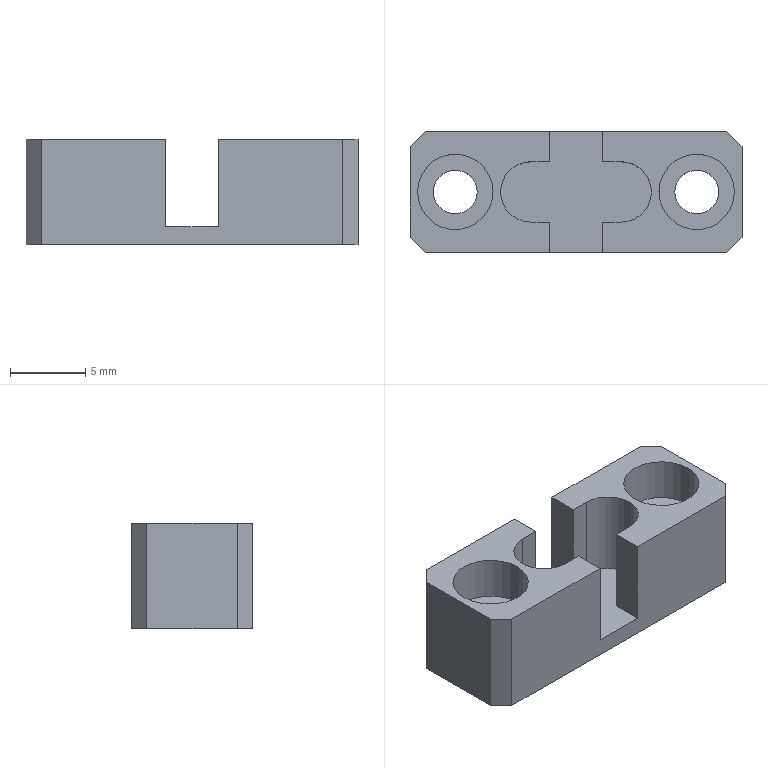Part | SolidWorks | features Chamfer 1, Extrusion 1, HoleWzd 1, ICE 1 | 1 solid | 33 faces | box 22 x 8 x 7 mm | volume 756.67 mm3 | plane 22 | cylinder 11 | commonest cylinder face diameters 2.9 x4 5 x4 4 x3
STEP:
#1=CARTESIAN_POINT('',(-10.5,0.,4.1));
#2=VERTEX_POINT('',#1);
#3=CARTESIAN_POINT('',(-5.5,0.,4.1));
#4=VERTEX_POINT('',#3);
#5=CARTESIAN_POINT('',(-8.,0.,4.1));
#6=DIRECTION('',(0.,0.,1.));
#7=DIRECTION('',(1.,0.,0.));
#8=AXIS2_PLACEMENT_3D('',#5,#6,#7);
#9=CIRCLE('',#8,2.5);
#10=EDGE_CURVE('',#2,#4,#9,.T.);
#11=ORIENTED_EDGE('',*,*,#10,.F.);
#12=CARTESIAN_POINT('',(-10.5,0.,7.));
#13=VERTEX_POINT('',#12);
#14=CARTESIAN_POINT('',(-10.5,0.,7.));
#15=DIRECTION('',(0.,0.,1.));
#16=VECTOR('',#15,1000.);
#17=LINE('',#14,#16);
#18=EDGE_CURVE('',#2,#13,#17,.T.);
#19=ORIENTED_EDGE('',*,*,#18,.T.);
#20=CARTESIAN_POINT('',(-5.5,0.,7.));
#21=VERTEX_POINT('',#20);
#22=CARTESIAN_POINT('',(-8.,0.,7.));
#23=DIRECTION('',(0.,0.,1.));
#24=DIRECTION('',(1.,0.,0.));
#25=AXIS2_PLACEMENT_3D('',#22,#23,#24);
#26=CIRCLE('',#25,2.5);
#27=EDGE_CURVE('',#13,#21,#26,.T.);
#28=ORIENTED_EDGE('',*,*,#27,.T.);
#29=CARTESIAN_POINT('',(-5.5,0.,7.));
#30=DIRECTION('',(0.,0.,1.));
#31=VECTOR('',#30,1000.);
#32=LINE('',#29,#31);
#33=EDGE_CURVE('',#4,#21,#32,.T.);
#34=ORIENTED_EDGE('',*,*,#33,.F.);
#35=EDGE_LOOP('',(#11,#19,#28,#34));
#36=FACE_OUTER_BOUND('',#35,.T.);
#37=CARTESIAN_POINT('',(-8.,0.,7.));
#38=DIRECTION('',(0.,0.,1.));
#39=DIRECTION('',(1.,0.,0.));
#40=AXIS2_PLACEMENT_3D('',#37,#38,#39);
#41=CYLINDRICAL_SURFACE('',#40,2.5);
#42=ADVANCED_FACE('',(#36),#41,.F.);
#43=CARTESIAN_POINT('',(-9.45,0.,0.));
#44=VERTEX_POINT('',#43);
#45=CARTESIAN_POINT('',(-6.55,0.,0.));
#46=VERTEX_POINT('',#45);
#47=CARTESIAN_POINT('',(-8.,0.,0.));
#48=DIRECTION('',(0.,0.,1.));
#49=DIRECTION('',(1.,0.,0.));
#50=AXIS2_PLACEMENT_3D('',#47,#48,#49);
#51=CIRCLE('',#50,1.45);
#52=EDGE_CURVE('',#44,#46,#51,.T.);
#53=ORIENTED_EDGE('',*,*,#52,.F.);
#54=CARTESIAN_POINT('',(-9.45,0.,4.1));
#55=VERTEX_POINT('',#54);
#56=CARTESIAN_POINT('',(-9.45,0.,7.));
#57=DIRECTION('',(0.,0.,1.));
#58=VECTOR('',#57,1000.);
#59=LINE('',#56,#58);
#60=EDGE_CURVE('',#44,#55,#59,.T.);
#61=ORIENTED_EDGE('',*,*,#60,.T.);
#62=CARTESIAN_POINT('',(-6.55,0.,4.1));
#63=VERTEX_POINT('',#62);
#64=CARTESIAN_POINT('',(-8.,0.,4.1));
#65=DIRECTION('',(0.,0.,1.));
#66=DIRECTION('',(1.,0.,0.));
#67=AXIS2_PLACEMENT_3D('',#64,#65,#66);
#68=CIRCLE('',#67,1.45);
#69=EDGE_CURVE('',#55,#63,#68,.T.);
#70=ORIENTED_EDGE('',*,*,#69,.T.);
#71=CARTESIAN_POINT('',(-6.55,0.,7.));
#72=DIRECTION('',(0.,0.,1.));
#73=VECTOR('',#72,1000.);
#74=LINE('',#71,#73);
#75=EDGE_CURVE('',#46,#63,#74,.T.);
#76=ORIENTED_EDGE('',*,*,#75,.F.);
#77=EDGE_LOOP('',(#53,#61,#70,#76));
#78=FACE_OUTER_BOUND('',#77,.T.);
#79=CARTESIAN_POINT('',(-8.,0.,7.));
#80=DIRECTION('',(0.,0.,1.));
#81=DIRECTION('',(1.,0.,0.));
#82=AXIS2_PLACEMENT_3D('',#79,#80,#81);
#83=CYLINDRICAL_SURFACE('',#82,1.45);
#84=ADVANCED_FACE('',(#78),#83,.F.);
#85=CARTESIAN_POINT('',(5.5,0.,4.1));
#86=VERTEX_POINT('',#85);
#87=CARTESIAN_POINT('',(10.5,0.,4.1));
#88=VERTEX_POINT('',#87);
#89=CARTESIAN_POINT('',(8.,0.,4.1));
#90=DIRECTION('',(0.,0.,1.));
#91=DIRECTION('',(1.,0.,0.));
#92=AXIS2_PLACEMENT_3D('',#89,#90,#91);
#93=CIRCLE('',#92,2.5);
#94=EDGE_CURVE('',#86,#88,#93,.T.);
#95=ORIENTED_EDGE('',*,*,#94,.F.);
#96=CARTESIAN_POINT('',(5.5,0.,7.));
#97=VERTEX_POINT('',#96);
#98=CARTESIAN_POINT('',(5.5,0.,7.));
#99=DIRECTION('',(0.,0.,1.));
#100=VECTOR('',#99,1000.);
#101=LINE('',#98,#100);
#102=EDGE_CURVE('',#86,#97,#101,.T.);
#103=ORIENTED_EDGE('',*,*,#102,.T.);
#104=CARTESIAN_POINT('',(10.5,0.,7.));
#105=VERTEX_POINT('',#104);
#106=CARTESIAN_POINT('',(8.,0.,7.));
#107=DIRECTION('',(0.,0.,1.));
#108=DIRECTION('',(1.,0.,0.));
#109=AXIS2_PLACEMENT_3D('',#106,#107,#108);
#110=CIRCLE('',#109,2.5);
#111=EDGE_CURVE('',#97,#105,#110,.T.);
#112=ORIENTED_EDGE('',*,*,#111,.T.);
#113=CARTESIAN_POINT('',(10.5,0.,7.));
#114=DIRECTION('',(0.,0.,1.));
#115=VECTOR('',#114,1000.);
#116=LINE('',#113,#115);
#117=EDGE_CURVE('',#88,#105,#116,.T.);
#118=ORIENTED_EDGE('',*,*,#117,.F.);
#119=EDGE_LOOP('',(#95,#103,#112,#118));
#120=FACE_OUTER_BOUND('',#119,.T.);
#121=CARTESIAN_POINT('',(8.,0.,7.));
#122=DIRECTION('',(0.,0.,1.));
#123=DIRECTION('',(1.,0.,0.));
#124=AXIS2_PLACEMENT_3D('',#121,#122,#123);
#125=CYLINDRICAL_SURFACE('',#124,2.5);
#126=ADVANCED_FACE('',(#120),#125,.F.);
#127=CARTESIAN_POINT('',(6.55,0.,0.));
#128=VERTEX_POINT('',#127);
#129=CARTESIAN_POINT('',(9.45,0.,0.));
#130=VERTEX_POINT('',#129);
#131=CARTESIAN_POINT('',(8.,0.,0.));
#132=DIRECTION('',(0.,0.,1.));
#133=DIRECTION('',(1.,0.,0.));
#134=AXIS2_PLACEMENT_3D('',#131,#132,#133);
#135=CIRCLE('',#134,1.45);
#136=EDGE_CURVE('',#128,#130,#135,.T.);
#137=ORIENTED_EDGE('',*,*,#136,.F.);
#138=CARTESIAN_POINT('',(6.55,0.,4.1));
#139=VERTEX_POINT('',#138);
#140=CARTESIAN_POINT('',(6.55,0.,7.));
#141=DIRECTION('',(0.,0.,1.));
#142=VECTOR('',#141,1000.);
#143=LINE('',#140,#142);
#144=EDGE_CURVE('',#128,#139,#143,.T.);
#145=ORIENTED_EDGE('',*,*,#144,.T.);
#146=CARTESIAN_POINT('',(9.45,0.,4.1));
#147=VERTEX_POINT('',#146);
#148=CARTESIAN_POINT('',(8.,0.,4.1));
#149=DIRECTION('',(0.,0.,1.));
#150=DIRECTION('',(1.,0.,0.));
#151=AXIS2_PLACEMENT_3D('',#148,#149,#150);
#152=CIRCLE('',#151,1.45);
#153=EDGE_CURVE('',#139,#147,#152,.T.);
#154=ORIENTED_EDGE('',*,*,#153,.T.);
#155=CARTESIAN_POINT('',(9.45,0.,7.));
#156=DIRECTION('',(0.,0.,1.));
#157=VECTOR('',#156,1000.);
#158=LINE('',#155,#157);
#159=EDGE_CURVE('',#130,#147,#158,.T.);
#160=ORIENTED_EDGE('',*,*,#159,.F.);
#161=EDGE_LOOP('',(#137,#145,#154,#160));
#162=FACE_OUTER_BOUND('',#161,.T.);
#163=CARTESIAN_POINT('',(8.,0.,7.));
#164=DIRECTION('',(0.,0.,1.));
#165=DIRECTION('',(1.,0.,0.));
#166=AXIS2_PLACEMENT_3D('',#163,#164,#165);
#167=CYLINDRICAL_SURFACE('',#166,1.45);
#168=ADVANCED_FACE('',(#162),#167,.F.);
#169=CARTESIAN_POINT('',(5.,0.,1.2));
#170=VERTEX_POINT('',#169);
#171=CARTESIAN_POINT('',(3.,2.,1.2));
#172=VERTEX_POINT('',#171);
#173=CARTESIAN_POINT('',(3.,0.,1.2));
#174=DIRECTION('',(0.,0.,1.));
#175=DIRECTION('',(-1.,0.,0.));
#176=AXIS2_PLACEMENT_3D('',#173,#174,#175);
#177=CIRCLE('',#176,2.);
#178=EDGE_CURVE('',#170,#172,#177,.T.);
#179=ORIENTED_EDGE('',*,*,#178,.F.);
#180=CARTESIAN_POINT('',(5.,0.,7.));
#181=VERTEX_POINT('',#180);
#182=CARTESIAN_POINT('',(5.,0.,1.2));
#183=DIRECTION('',(0.,0.,1.));
#184=VECTOR('',#183,1000.);
#185=LINE('',#182,#184);
#186=EDGE_CURVE('',#170,#181,#185,.T.);
#187=ORIENTED_EDGE('',*,*,#186,.T.);
#188=CARTESIAN_POINT('',(3.,2.,7.));
#189=VERTEX_POINT('',#188);
#190=CARTESIAN_POINT('',(3.,0.,7.));
#191=DIRECTION('',(0.,0.,1.));
#192=DIRECTION('',(-1.,0.,0.));
#193=AXIS2_PLACEMENT_3D('',#190,#191,#192);
#194=CIRCLE('',#193,2.);
#195=EDGE_CURVE('',#181,#189,#194,.T.);
#196=ORIENTED_EDGE('',*,*,#195,.T.);
#197=CARTESIAN_POINT('',(3.,2.,1.2));
#198=DIRECTION('',(0.,0.,1.));
#199=VECTOR('',#198,1000.);
#200=LINE('',#197,#199);
#201=EDGE_CURVE('',#172,#189,#200,.T.);
#202=ORIENTED_EDGE('',*,*,#201,.F.);
#203=EDGE_LOOP('',(#179,#187,#196,#202));
#204=FACE_OUTER_BOUND('',#203,.T.);
#205=CARTESIAN_POINT('',(3.,0.,1.2));
#206=DIRECTION('',(0.,0.,1.));
#207=DIRECTION('',(1.,0.,0.));
#208=AXIS2_PLACEMENT_3D('',#205,#206,#207);
#209=CYLINDRICAL_SURFACE('',#208,2.);
#210=ADVANCED_FACE('',(#204),#209,.F.);
#211=CARTESIAN_POINT('',(8.,0.,7.));
#212=DIRECTION('',(0.,0.,1.));
#213=DIRECTION('',(1.,0.,0.));
#214=AXIS2_PLACEMENT_3D('',#211,#212,#213);
#215=CIRCLE('',#214,2.5);
#216=EDGE_CURVE('',#105,#97,#215,.T.);
#217=ORIENTED_EDGE('',*,*,#216,.F.);
#218=ORIENTED_EDGE('',*,*,#111,.F.);
#219=EDGE_LOOP('',(#217,#218));
#220=FACE_BOUND('',#219,.T.);
#221=CARTESIAN_POINT('',(1.75,-4.,7.));
#222=VERTEX_POINT('',#221);
#223=CARTESIAN_POINT('',(10.,-4.,7.));
#224=VERTEX_POINT('',#223);
#225=CARTESIAN_POINT('',(-11.,-4.,7.));
#226=DIRECTION('',(1.,0.,0.));
#227=VECTOR('',#226,1000.);
#228=LINE('',#225,#227);
#229=EDGE_CURVE('',#222,#224,#228,.T.);
#230=ORIENTED_EDGE('',*,*,#229,.T.);
#231=CARTESIAN_POINT('',(11.,-3.,7.));
#232=VERTEX_POINT('',#231);
#233=CARTESIAN_POINT('',(11.,-3.,7.));
#234=DIRECTION('',(0.7071,0.7071,0.));
#235=VECTOR('',#234,1000.);
#236=LINE('',#233,#235);
#237=EDGE_CURVE('',#224,#232,#236,.T.);
#238=ORIENTED_EDGE('',*,*,#237,.T.);
#239=CARTESIAN_POINT('',(11.,3.,7.));
#240=VERTEX_POINT('',#239);
#241=CARTESIAN_POINT('',(11.,-4.,7.));
#242=DIRECTION('',(0.,1.,0.));
#243=VECTOR('',#242,1000.);
#244=LINE('',#241,#243);
#245=EDGE_CURVE('',#232,#240,#244,.T.);
#246=ORIENTED_EDGE('',*,*,#245,.T.);
#247=CARTESIAN_POINT('',(10.,4.,7.));
#248=VERTEX_POINT('',#247);
#249=CARTESIAN_POINT('',(10.,4.,7.));
#250=DIRECTION('',(-0.7071,0.7071,0.));
#251=VECTOR('',#250,1000.);
#252=LINE('',#249,#251);
#253=EDGE_CURVE('',#240,#248,#252,.T.);
#254=ORIENTED_EDGE('',*,*,#253,.T.);
#255=CARTESIAN_POINT('',(1.75,4.,7.));
#256=VERTEX_POINT('',#255);
#257=CARTESIAN_POINT('',(-11.,4.,7.));
#258=DIRECTION('',(-1.,0.,0.));
#259=VECTOR('',#258,1000.);
#260=LINE('',#257,#259);
#261=EDGE_CURVE('',#248,#256,#260,.T.);
#262=ORIENTED_EDGE('',*,*,#261,.T.);
#263=CARTESIAN_POINT('',(1.75,2.,7.));
#264=VERTEX_POINT('',#263);
#265=CARTESIAN_POINT('',(1.75,4.,7.));
#266=DIRECTION('',(0.,1.,0.));
#267=VECTOR('',#266,1000.);
#268=LINE('',#265,#267);
#269=EDGE_CURVE('',#264,#256,#268,.T.);
#270=ORIENTED_EDGE('',*,*,#269,.F.);
#271=CARTESIAN_POINT('',(1.75,2.,7.));
#272=DIRECTION('',(-1.,0.,0.));
#273=VECTOR('',#272,1000.);
#274=LINE('',#271,#273);
#275=EDGE_CURVE('',#189,#264,#274,.T.);
#276=ORIENTED_EDGE('',*,*,#275,.F.);
#277=ORIENTED_EDGE('',*,*,#195,.F.);
#278=CARTESIAN_POINT('',(3.,-2.,7.));
#279=VERTEX_POINT('',#278);
#280=CARTESIAN_POINT('',(3.,0.,7.));
#281=DIRECTION('',(0.,0.,1.));
#282=DIRECTION('',(-1.,0.,0.));
#283=AXIS2_PLACEMENT_3D('',#280,#281,#282);
#284=CIRCLE('',#283,2.);
#285=EDGE_CURVE('',#279,#181,#284,.T.);
#286=ORIENTED_EDGE('',*,*,#285,.F.);
#287=CARTESIAN_POINT('',(1.75,-2.,7.));
#288=VERTEX_POINT('',#287);
#289=CARTESIAN_POINT('',(1.75,-2.,7.));
#290=DIRECTION('',(1.,0.,0.));
#291=VECTOR('',#290,1000.);
#292=LINE('',#289,#291);
#293=EDGE_CURVE('',#288,#279,#292,.T.);
#294=ORIENTED_EDGE('',*,*,#293,.F.);
#295=CARTESIAN_POINT('',(1.75,-2.,7.));
#296=DIRECTION('',(0.,1.,0.));
#297=VECTOR('',#296,1000.);
#298=LINE('',#295,#297);
#299=EDGE_CURVE('',#222,#288,#298,.T.);
#300=ORIENTED_EDGE('',*,*,#299,.F.);
#301=EDGE_LOOP('',(#230,#238,#246,#254,#262,#270,#276,#277,#286,#294,#300));
#302=FACE_OUTER_BOUND('',#301,.T.);
#303=CARTESIAN_POINT('',(0.,0.,7.));
#304=DIRECTION('',(0.,0.,-1.));
#305=DIRECTION('',(-1.,0.,0.));
#306=AXIS2_PLACEMENT_3D('',#303,#304,#305);
#307=PLANE('',#306);
#308=ADVANCED_FACE('',(#220,#302),#307,.F.);
#309=ORIENTED_EDGE('',*,*,#245,.F.);
#310=CARTESIAN_POINT('',(11.,-3.,0.));
#311=VERTEX_POINT('',#310);
#312=CARTESIAN_POINT('',(11.,-3.,7.));
#313=DIRECTION('',(0.,0.,-1.));
#314=VECTOR('',#313,1000.);
#315=LINE('',#312,#314);
#316=EDGE_CURVE('',#232,#311,#315,.T.);
#317=ORIENTED_EDGE('',*,*,#316,.T.);
#318=CARTESIAN_POINT('',(11.,3.,0.));
#319=VERTEX_POINT('',#318);
#320=CARTESIAN_POINT('',(11.,-4.,0.));
#321=DIRECTION('',(0.,1.,0.));
#322=VECTOR('',#321,1000.);
#323=LINE('',#320,#322);
#324=EDGE_CURVE('',#311,#319,#323,.T.);
#325=ORIENTED_EDGE('',*,*,#324,.T.);
#326=CARTESIAN_POINT('',(11.,3.,7.));
#327=DIRECTION('',(0.,0.,1.));
#328=VECTOR('',#327,1000.);
#329=LINE('',#326,#328);
#330=EDGE_CURVE('',#319,#240,#329,.T.);
#331=ORIENTED_EDGE('',*,*,#330,.T.);
#332=EDGE_LOOP('',(#309,#317,#325,#331));
#333=FACE_OUTER_BOUND('',#332,.T.);
#334=CARTESIAN_POINT('',(11.,-4.,7.));
#335=DIRECTION('',(-1.,0.,0.));
#336=DIRECTION('',(0.,0.,1.));
#337=AXIS2_PLACEMENT_3D('',#334,#335,#336);
#338=PLANE('',#337);
#339=ADVANCED_FACE('',(#333),#338,.F.);
#340=ORIENTED_EDGE('',*,*,#261,.F.);
#341=CARTESIAN_POINT('',(10.,4.,0.));
#342=VERTEX_POINT('',#341);
#343=CARTESIAN_POINT('',(10.,4.,7.));
#344=DIRECTION('',(0.,0.,-1.));
#345=VECTOR('',#344,1000.);
#346=LINE('',#343,#345);
#347=EDGE_CURVE('',#248,#342,#346,.T.);
#348=ORIENTED_EDGE('',*,*,#347,.T.);
#349=CARTESIAN_POINT('',(-10.,4.,0.));
#350=VERTEX_POINT('',#349);
#351=CARTESIAN_POINT('',(-11.,4.,0.));
#352=DIRECTION('',(-1.,0.,0.));
#353=VECTOR('',#352,1000.);
#354=LINE('',#351,#353);
#355=EDGE_CURVE('',#342,#350,#354,.T.);
#356=ORIENTED_EDGE('',*,*,#355,.T.);
#357=CARTESIAN_POINT('',(-10.,4.,7.));
#358=VERTEX_POINT('',#357);
#359=CARTESIAN_POINT('',(-10.,4.,7.));
#360=DIRECTION('',(0.,0.,1.));
#361=VECTOR('',#360,1000.);
#362=LINE('',#359,#361);
#363=EDGE_CURVE('',#350,#358,#362,.T.);
#364=ORIENTED_EDGE('',*,*,#363,.T.);
#365=CARTESIAN_POINT('',(-1.75,4.,7.));
#366=VERTEX_POINT('',#365);
#367=CARTESIAN_POINT('',(-11.,4.,7.));
#368=DIRECTION('',(-1.,0.,0.));
#369=VECTOR('',#368,1000.);
#370=LINE('',#367,#369);
#371=EDGE_CURVE('',#366,#358,#370,.T.);
#372=ORIENTED_EDGE('',*,*,#371,.F.);
#373=CARTESIAN_POINT('',(-1.75,4.,1.2));
#374=VERTEX_POINT('',#373);
#375=CARTESIAN_POINT('',(-1.75,4.,1.2));
#376=DIRECTION('',(0.,0.,1.));
#377=VECTOR('',#376,1000.);
#378=LINE('',#375,#377);
#379=EDGE_CURVE('',#374,#366,#378,.T.);
#380=ORIENTED_EDGE('',*,*,#379,.F.);
#381=CARTESIAN_POINT('',(1.75,4.,1.2));
#382=VERTEX_POINT('',#381);
#383=CARTESIAN_POINT('',(-1.75,4.,1.2));
#384=DIRECTION('',(-1.,0.,0.));
#385=VECTOR('',#384,1000.);
#386=LINE('',#383,#385);
#387=EDGE_CURVE('',#382,#374,#386,.T.);
#388=ORIENTED_EDGE('',*,*,#387,.F.);
#389=CARTESIAN_POINT('',(1.75,4.,1.2));
#390=DIRECTION('',(0.,0.,1.));
#391=VECTOR('',#390,1000.);
#392=LINE('',#389,#391);
#393=EDGE_CURVE('',#382,#256,#392,.T.);
#394=ORIENTED_EDGE('',*,*,#393,.T.);
#395=EDGE_LOOP('',(#340,#348,#356,#364,#372,#380,#388,#394));
#396=FACE_OUTER_BOUND('',#395,.T.);
#397=CARTESIAN_POINT('',(-11.,4.,7.));
#398=DIRECTION('',(0.,-1.,0.));
#399=DIRECTION('',(0.,0.,-1.));
#400=AXIS2_PLACEMENT_3D('',#397,#398,#399);
#401=PLANE('',#400);
#402=ADVANCED_FACE('',(#396),#401,.F.);
#403=CARTESIAN_POINT('',(-11.,3.,0.));
#404=VERTEX_POINT('',#403);
#405=CARTESIAN_POINT('',(-11.,-3.,0.));
#406=VERTEX_POINT('',#405);
#407=CARTESIAN_POINT('',(-11.,-4.,0.));
#408=DIRECTION('',(0.,-1.,0.));
#409=VECTOR('',#408,1000.);
#410=LINE('',#407,#409);
#411=EDGE_CURVE('',#404,#406,#410,.T.);
#412=ORIENTED_EDGE('',*,*,#411,.T.);
#413=CARTESIAN_POINT('',(-11.,-3.,7.));
#414=VERTEX_POINT('',#413);
#415=CARTESIAN_POINT('',(-11.,-3.,7.));
#416=DIRECTION('',(0.,0.,1.));
#417=VECTOR('',#416,1000.);
#418=LINE('',#415,#417);
#419=EDGE_CURVE('',#406,#414,#418,.T.);
#420=ORIENTED_EDGE('',*,*,#419,.T.);
#421=CARTESIAN_POINT('',(-11.,3.,7.));
#422=VERTEX_POINT('',#421);
#423=CARTESIAN_POINT('',(-11.,-4.,7.));
#424=DIRECTION('',(0.,-1.,0.));
#425=VECTOR('',#424,1000.);
#426=LINE('',#423,#425);
#427=EDGE_CURVE('',#422,#414,#426,.T.);
#428=ORIENTED_EDGE('',*,*,#427,.F.);
#429=CARTESIAN_POINT('',(-11.,3.,7.));
#430=DIRECTION('',(0.,0.,-1.));
#431=VECTOR('',#430,1000.);
#432=LINE('',#429,#431);
#433=EDGE_CURVE('',#422,#404,#432,.T.);
#434=ORIENTED_EDGE('',*,*,#433,.T.);
#435=EDGE_LOOP('',(#412,#420,#428,#434));
#436=FACE_OUTER_BOUND('',#435,.T.);
#437=CARTESIAN_POINT('',(-11.,-4.,7.));
#438=DIRECTION('',(1.,0.,0.));
#439=DIRECTION('',(0.,0.,-1.));
#440=AXIS2_PLACEMENT_3D('',#437,#438,#439);
#441=PLANE('',#440);
#442=ADVANCED_FACE('',(#436),#441,.F.);
#443=CARTESIAN_POINT('',(-10.,-4.,0.));
#444=VERTEX_POINT('',#443);
#445=CARTESIAN_POINT('',(10.,-4.,0.));
#446=VERTEX_POINT('',#445);
#447=CARTESIAN_POINT('',(-11.,-4.,0.));
#448=DIRECTION('',(1.,0.,0.));
#449=VECTOR('',#448,1000.);
#450=LINE('',#447,#449);
#451=EDGE_CURVE('',#444,#446,#450,.T.);
#452=ORIENTED_EDGE('',*,*,#451,.T.);
#453=CARTESIAN_POINT('',(10.,-4.,7.));
#454=DIRECTION('',(0.,0.,1.));
#455=VECTOR('',#454,1000.);
#456=LINE('',#453,#455);
#457=EDGE_CURVE('',#446,#224,#456,.T.);
#458=ORIENTED_EDGE('',*,*,#457,.T.);
#459=ORIENTED_EDGE('',*,*,#229,.F.);
#460=CARTESIAN_POINT('',(1.75,-4.,1.2));
#461=VERTEX_POINT('',#460);
#462=CARTESIAN_POINT('',(1.75,-4.,1.2));
#463=DIRECTION('',(0.,0.,1.));
#464=VECTOR('',#463,1000.);
#465=LINE('',#462,#464);
#466=EDGE_CURVE('',#461,#222,#465,.T.);
#467=ORIENTED_EDGE('',*,*,#466,.F.);
#468=CARTESIAN_POINT('',(-1.75,-4.,1.2));
#469=VERTEX_POINT('',#468);
#470=CARTESIAN_POINT('',(-1.75,-4.,1.2));
#471=DIRECTION('',(1.,0.,0.));
#472=VECTOR('',#471,1000.);
#473=LINE('',#470,#472);
#474=EDGE_CURVE('',#469,#461,#473,.T.);
#475=ORIENTED_EDGE('',*,*,#474,.F.);
#476=CARTESIAN_POINT('',(-1.75,-4.,7.));
#477=VERTEX_POINT('',#476);
#478=CARTESIAN_POINT('',(-1.75,-4.,1.2));
#479=DIRECTION('',(0.,0.,1.));
#480=VECTOR('',#479,1000.);
#481=LINE('',#478,#480);
#482=EDGE_CURVE('',#469,#477,#481,.T.);
#483=ORIENTED_EDGE('',*,*,#482,.T.);
#484=CARTESIAN_POINT('',(-10.,-4.,7.));
#485=VERTEX_POINT('',#484);
#486=CARTESIAN_POINT('',(-11.,-4.,7.));
#487=DIRECTION('',(1.,0.,0.));
#488=VECTOR('',#487,1000.);
#489=LINE('',#486,#488);
#490=EDGE_CURVE('',#485,#477,#489,.T.);
#491=ORIENTED_EDGE('',*,*,#490,.F.);
#492=CARTESIAN_POINT('',(-10.,-4.,7.));
#493=DIRECTION('',(0.,0.,-1.));
#494=VECTOR('',#493,1000.);
#495=LINE('',#492,#494);
#496=EDGE_CURVE('',#485,#444,#495,.T.);
#497=ORIENTED_EDGE('',*,*,#496,.T.);
#498=EDGE_LOOP('',(#452,#458,#459,#467,#475,#483,#491,#497));
#499=FACE_OUTER_BOUND('',#498,.T.);
#500=CARTESIAN_POINT('',(-11.,-4.,7.));
#501=DIRECTION('',(0.,1.,0.));
#502=DIRECTION('',(0.,0.,1.));
#503=AXIS2_PLACEMENT_3D('',#500,#501,#502);
#504=PLANE('',#503);
#505=ADVANCED_FACE('',(#499),#504,.F.);
#506=CARTESIAN_POINT('',(-8.,0.,7.));
#507=DIRECTION('',(0.,0.,1.));
#508=DIRECTION('',(1.,0.,0.));
#509=AXIS2_PLACEMENT_3D('',#506,#507,#508);
#510=CIRCLE('',#509,2.5);
#511=EDGE_CURVE('',#21,#13,#510,.T.);
#512=ORIENTED_EDGE('',*,*,#511,.F.);
#513=ORIENTED_EDGE('',*,*,#27,.F.);
#514=EDGE_LOOP('',(#512,#513));
#515=FACE_BOUND('',#514,.T.);
#516=ORIENTED_EDGE('',*,*,#427,.T.);
#517=CARTESIAN_POINT('',(-10.,-4.,7.));
#518=DIRECTION('',(0.7071,-0.7071,0.));
#519=VECTOR('',#518,1000.);
#520=LINE('',#517,#519);
#521=EDGE_CURVE('',#414,#485,#520,.T.);
#522=ORIENTED_EDGE('',*,*,#521,.T.);
#523=ORIENTED_EDGE('',*,*,#490,.T.);
#524=CARTESIAN_POINT('',(-1.75,-2.,7.));
#525=VERTEX_POINT('',#524);
#526=CARTESIAN_POINT('',(-1.75,-2.,7.));
#527=DIRECTION('',(0.,-1.,0.));
#528=VECTOR('',#527,1000.);
#529=LINE('',#526,#528);
#530=EDGE_CURVE('',#525,#477,#529,.T.);
#531=ORIENTED_EDGE('',*,*,#530,.F.);
#532=CARTESIAN_POINT('',(-3.,-2.,7.));
#533=VERTEX_POINT('',#532);
#534=CARTESIAN_POINT('',(-3.,-2.,7.));
#535=DIRECTION('',(1.,0.,0.));
#536=VECTOR('',#535,1000.);
#537=LINE('',#534,#536);
#538=EDGE_CURVE('',#533,#525,#537,.T.);
#539=ORIENTED_EDGE('',*,*,#538,.F.);
#540=CARTESIAN_POINT('',(-3.,2.,7.));
#541=VERTEX_POINT('',#540);
#542=CARTESIAN_POINT('',(-3.,0.,7.));
#543=DIRECTION('',(0.,0.,1.));
#544=DIRECTION('',(1.,0.,0.));
#545=AXIS2_PLACEMENT_3D('',#542,#543,#544);
#546=CIRCLE('',#545,2.);
#547=EDGE_CURVE('',#541,#533,#546,.T.);
#548=ORIENTED_EDGE('',*,*,#547,.F.);
#549=CARTESIAN_POINT('',(-1.75,2.,7.));
#550=VERTEX_POINT('',#549);
#551=CARTESIAN_POINT('',(-3.,2.,7.));
#552=DIRECTION('',(-1.,0.,0.));
#553=VECTOR('',#552,1000.);
#554=LINE('',#551,#553);
#555=EDGE_CURVE('',#550,#541,#554,.T.);
#556=ORIENTED_EDGE('',*,*,#555,.F.);
#557=CARTESIAN_POINT('',(-1.75,4.,7.));
#558=DIRECTION('',(0.,-1.,0.));
#559=VECTOR('',#558,1000.);
#560=LINE('',#557,#559);
#561=EDGE_CURVE('',#366,#550,#560,.T.);
#562=ORIENTED_EDGE('',*,*,#561,.F.);
#563=ORIENTED_EDGE('',*,*,#371,.T.);
#564=CARTESIAN_POINT('',(-11.,3.,7.));
#565=DIRECTION('',(-0.7071,-0.7071,0.));
#566=VECTOR('',#565,1000.);
#567=LINE('',#564,#566);
#568=EDGE_CURVE('',#358,#422,#567,.T.);
#569=ORIENTED_EDGE('',*,*,#568,.T.);
#570=EDGE_LOOP('',(#516,#522,#523,#531,#539,#548,#556,#562,#563,#569));
#571=FACE_OUTER_BOUND('',#570,.T.);
#572=CARTESIAN_POINT('',(0.,0.,7.));
#573=DIRECTION('',(0.,0.,-1.));
#574=DIRECTION('',(-1.,0.,0.));
#575=AXIS2_PLACEMENT_3D('',#572,#573,#574);
#576=PLANE('',#575);
#577=ADVANCED_FACE('',(#515,#571),#576,.F.);
#578=CARTESIAN_POINT('',(-8.,0.,0.));
#579=DIRECTION('',(0.,0.,1.));
#580=DIRECTION('',(1.,0.,0.));
#581=AXIS2_PLACEMENT_3D('',#578,#579,#580);
#582=CIRCLE('',#581,1.45);
#583=EDGE_CURVE('',#46,#44,#582,.T.);
#584=ORIENTED_EDGE('',*,*,#583,.T.);
#585=ORIENTED_EDGE('',*,*,#52,.T.);
#586=EDGE_LOOP('',(#584,#585));
#587=FACE_BOUND('',#586,.T.);
#588=CARTESIAN_POINT('',(8.,0.,0.));
#589=DIRECTION('',(0.,0.,1.));
#590=DIRECTION('',(1.,0.,0.));
#591=AXIS2_PLACEMENT_3D('',#588,#589,#590);
#592=CIRCLE('',#591,1.45);
#593=EDGE_CURVE('',#130,#128,#592,.T.);
#594=ORIENTED_EDGE('',*,*,#593,.T.);
#595=ORIENTED_EDGE('',*,*,#136,.T.);
#596=EDGE_LOOP('',(#594,#595));
#597=FACE_BOUND('',#596,.T.);
#598=ORIENTED_EDGE('',*,*,#324,.F.);
#599=CARTESIAN_POINT('',(7.,-7.,0.));
#600=DIRECTION('',(-0.7071,-0.7071,0.));
#601=VECTOR('',#600,1000.);
#602=LINE('',#599,#601);
#603=EDGE_CURVE('',#311,#446,#602,.T.);
#604=ORIENTED_EDGE('',*,*,#603,.T.);
#605=ORIENTED_EDGE('',*,*,#451,.F.);
#606=CARTESIAN_POINT('',(-7.,-7.,0.));
#607=DIRECTION('',(-0.7071,0.7071,0.));
#608=VECTOR('',#607,1000.);
#609=LINE('',#606,#608);
#610=EDGE_CURVE('',#444,#406,#609,.T.);
#611=ORIENTED_EDGE('',*,*,#610,.T.);
#612=ORIENTED_EDGE('',*,*,#411,.F.);
#613=CARTESIAN_POINT('',(-7.,7.,0.));
#614=DIRECTION('',(0.7071,0.7071,0.));
#615=VECTOR('',#614,1000.);
#616=LINE('',#613,#615);
#617=EDGE_CURVE('',#404,#350,#616,.T.);
#618=ORIENTED_EDGE('',*,*,#617,.T.);
#619=ORIENTED_EDGE('',*,*,#355,.F.);
#620=CARTESIAN_POINT('',(7.,7.,0.));
#621=DIRECTION('',(0.7071,-0.7071,0.));
#622=VECTOR('',#621,1000.);
#623=LINE('',#620,#622);
#624=EDGE_CURVE('',#342,#319,#623,.T.);
#625=ORIENTED_EDGE('',*,*,#624,.T.);
#626=EDGE_LOOP('',(#598,#604,#605,#611,#612,#618,#619,#625));
#627=FACE_OUTER_BOUND('',#626,.T.);
#628=CARTESIAN_POINT('',(0.,0.,0.));
#629=DIRECTION('',(0.,0.,-1.));
#630=DIRECTION('',(-1.,0.,0.));
#631=AXIS2_PLACEMENT_3D('',#628,#629,#630);
#632=PLANE('',#631);
#633=ADVANCED_FACE('',(#587,#597,#627),#632,.T.);
#634=ORIENTED_EDGE('',*,*,#561,.T.);
#635=CARTESIAN_POINT('',(-1.75,2.,1.2));
#636=VERTEX_POINT('',#635);
#637=CARTESIAN_POINT('',(-1.75,2.,1.2));
#638=DIRECTION('',(0.,0.,1.));
#639=VECTOR('',#638,1000.);
#640=LINE('',#637,#639);
#641=EDGE_CURVE('',#636,#550,#640,.T.);
#642=ORIENTED_EDGE('',*,*,#641,.F.);
#643=CARTESIAN_POINT('',(-1.75,4.,1.2));
#644=DIRECTION('',(0.,-1.,0.));
#645=VECTOR('',#644,1000.);
#646=LINE('',#643,#645);
#647=EDGE_CURVE('',#374,#636,#646,.T.);
#648=ORIENTED_EDGE('',*,*,#647,.F.);
#649=ORIENTED_EDGE('',*,*,#379,.T.);
#650=EDGE_LOOP('',(#634,#642,#648,#649));
#651=FACE_OUTER_BOUND('',#650,.T.);
#652=CARTESIAN_POINT('',(-1.75,4.,1.2));
#653=DIRECTION('',(-1.,0.,0.));
#654=DIRECTION('',(0.,-1.,0.));
#655=AXIS2_PLACEMENT_3D('',#652,#653,#654);
#656=PLANE('',#655);
#657=ADVANCED_FACE('',(#651),#656,.F.);
#658=ORIENTED_EDGE('',*,*,#269,.T.);
#659=ORIENTED_EDGE('',*,*,#393,.F.);
#660=CARTESIAN_POINT('',(1.75,2.,1.2));
#661=VERTEX_POINT('',#660);
#662=CARTESIAN_POINT('',(1.75,4.,1.2));
#663=DIRECTION('',(0.,1.,0.));
#664=VECTOR('',#663,1000.);
#665=LINE('',#662,#664);
#666=EDGE_CURVE('',#661,#382,#665,.T.);
#667=ORIENTED_EDGE('',*,*,#666,.F.);
#668=CARTESIAN_POINT('',(1.75,2.,1.2));
#669=DIRECTION('',(0.,0.,1.));
#670=VECTOR('',#669,1000.);
#671=LINE('',#668,#670);
#672=EDGE_CURVE('',#661,#264,#671,.T.);
#673=ORIENTED_EDGE('',*,*,#672,.T.);
#674=EDGE_LOOP('',(#658,#659,#667,#673));
#675=FACE_OUTER_BOUND('',#674,.T.);
#676=CARTESIAN_POINT('',(1.75,4.,1.2));
#677=DIRECTION('',(1.,0.,0.));
#678=DIRECTION('',(0.,1.,0.));
#679=AXIS2_PLACEMENT_3D('',#676,#677,#678);
#680=PLANE('',#679);
#681=ADVANCED_FACE('',(#675),#680,.F.);
#682=ORIENTED_EDGE('',*,*,#275,.T.);
#683=ORIENTED_EDGE('',*,*,#672,.F.);
#684=CARTESIAN_POINT('',(1.75,2.,1.2));
#685=DIRECTION('',(-1.,0.,0.));
#686=VECTOR('',#685,1000.);
#687=LINE('',#684,#686);
#688=EDGE_CURVE('',#172,#661,#687,.T.);
#689=ORIENTED_EDGE('',*,*,#688,.F.);
#690=ORIENTED_EDGE('',*,*,#201,.T.);
#691=EDGE_LOOP('',(#682,#683,#689,#690));
#692=FACE_OUTER_BOUND('',#691,.T.);
#693=CARTESIAN_POINT('',(1.75,2.,1.2));
#694=DIRECTION('',(0.,1.,0.));
#695=DIRECTION('',(-1.,0.,0.));
#696=AXIS2_PLACEMENT_3D('',#693,#694,#695);
#697=PLANE('',#696);
#698=ADVANCED_FACE('',(#692),#697,.F.);
#699=ORIENTED_EDGE('',*,*,#186,.F.);
#700=CARTESIAN_POINT('',(3.,-2.,1.2));
#701=VERTEX_POINT('',#700);
#702=CARTESIAN_POINT('',(3.,0.,1.2));
#703=DIRECTION('',(0.,0.,1.));
#704=DIRECTION('',(-1.,0.,0.));
#705=AXIS2_PLACEMENT_3D('',#702,#703,#704);
#706=CIRCLE('',#705,2.);
#707=EDGE_CURVE('',#701,#170,#706,.T.);
#708=ORIENTED_EDGE('',*,*,#707,.F.);
#709=CARTESIAN_POINT('',(3.,-2.,1.2));
#710=DIRECTION('',(0.,0.,1.));
#711=VECTOR('',#710,1000.);
#712=LINE('',#709,#711);
#713=EDGE_CURVE('',#701,#279,#712,.T.);
#714=ORIENTED_EDGE('',*,*,#713,.T.);
#715=ORIENTED_EDGE('',*,*,#285,.T.);
#716=EDGE_LOOP('',(#699,#708,#714,#715));
#717=FACE_OUTER_BOUND('',#716,.T.);
#718=CARTESIAN_POINT('',(3.,0.,1.2));
#719=DIRECTION('',(0.,0.,1.));
#720=DIRECTION('',(1.,0.,0.));
#721=AXIS2_PLACEMENT_3D('',#718,#719,#720);
#722=CYLINDRICAL_SURFACE('',#721,2.);
#723=ADVANCED_FACE('',(#717),#722,.F.);
#724=ORIENTED_EDGE('',*,*,#293,.T.);
#725=ORIENTED_EDGE('',*,*,#713,.F.);
#726=CARTESIAN_POINT('',(1.75,-2.,1.2));
#727=VERTEX_POINT('',#726);
#728=CARTESIAN_POINT('',(1.75,-2.,1.2));
#729=DIRECTION('',(1.,0.,0.));
#730=VECTOR('',#729,1000.);
#731=LINE('',#728,#730);
#732=EDGE_CURVE('',#727,#701,#731,.T.);
#733=ORIENTED_EDGE('',*,*,#732,.F.);
#734=CARTESIAN_POINT('',(1.75,-2.,1.2));
#735=DIRECTION('',(0.,0.,1.));
#736=VECTOR('',#735,1000.);
#737=LINE('',#734,#736);
#738=EDGE_CURVE('',#727,#288,#737,.T.);
#739=ORIENTED_EDGE('',*,*,#738,.T.);
#740=EDGE_LOOP('',(#724,#725,#733,#739));
#741=FACE_OUTER_BOUND('',#740,.T.);
#742=CARTESIAN_POINT('',(1.75,-2.,1.2));
#743=DIRECTION('',(0.,-1.,0.));
#744=DIRECTION('',(1.,0.,0.));
#745=AXIS2_PLACEMENT_3D('',#742,#743,#744);
#746=PLANE('',#745);
#747=ADVANCED_FACE('',(#741),#746,.F.);
#748=ORIENTED_EDGE('',*,*,#299,.T.);
#749=ORIENTED_EDGE('',*,*,#738,.F.);
#750=CARTESIAN_POINT('',(1.75,-2.,1.2));
#751=DIRECTION('',(0.,1.,0.));
#752=VECTOR('',#751,1000.);
#753=LINE('',#750,#752);
#754=EDGE_CURVE('',#461,#727,#753,.T.);
#755=ORIENTED_EDGE('',*,*,#754,.F.);
#756=ORIENTED_EDGE('',*,*,#466,.T.);
#757=EDGE_LOOP('',(#748,#749,#755,#756));
#758=FACE_OUTER_BOUND('',#757,.T.);
#759=CARTESIAN_POINT('',(1.75,-2.,1.2));
#760=DIRECTION('',(1.,0.,0.));
#761=DIRECTION('',(0.,1.,0.));
#762=AXIS2_PLACEMENT_3D('',#759,#760,#761);
#763=PLANE('',#762);
#764=ADVANCED_FACE('',(#758),#763,.F.);
#765=ORIENTED_EDGE('',*,*,#530,.T.);
#766=ORIENTED_EDGE('',*,*,#482,.F.);
#767=CARTESIAN_POINT('',(-1.75,-2.,1.2));
#768=VERTEX_POINT('',#767);
#769=CARTESIAN_POINT('',(-1.75,-2.,1.2));
#770=DIRECTION('',(0.,-1.,0.));
#771=VECTOR('',#770,1000.);
#772=LINE('',#769,#771);
#773=EDGE_CURVE('',#768,#469,#772,.T.);
#774=ORIENTED_EDGE('',*,*,#773,.F.);
#775=CARTESIAN_POINT('',(-1.75,-2.,1.2));
#776=DIRECTION('',(0.,0.,1.));
#777=VECTOR('',#776,1000.);
#778=LINE('',#775,#777);
#779=EDGE_CURVE('',#768,#525,#778,.T.);
#780=ORIENTED_EDGE('',*,*,#779,.T.);
#781=EDGE_LOOP('',(#765,#766,#774,#780));
#782=FACE_OUTER_BOUND('',#781,.T.);
#783=CARTESIAN_POINT('',(-1.75,-2.,1.2));
#784=DIRECTION('',(-1.,0.,0.));
#785=DIRECTION('',(0.,-1.,0.));
#786=AXIS2_PLACEMENT_3D('',#783,#784,#785);
#787=PLANE('',#786);
#788=ADVANCED_FACE('',(#782),#787,.F.);
#789=ORIENTED_EDGE('',*,*,#538,.T.);
#790=ORIENTED_EDGE('',*,*,#779,.F.);
#791=CARTESIAN_POINT('',(-3.,-2.,1.2));
#792=VERTEX_POINT('',#791);
#793=CARTESIAN_POINT('',(-3.,-2.,1.2));
#794=DIRECTION('',(1.,0.,0.));
#795=VECTOR('',#794,1000.);
#796=LINE('',#793,#795);
#797=EDGE_CURVE('',#792,#768,#796,.T.);
#798=ORIENTED_EDGE('',*,*,#797,.F.);
#799=CARTESIAN_POINT('',(-3.,-2.,1.2));
#800=DIRECTION('',(0.,0.,1.));
#801=VECTOR('',#800,1000.);
#802=LINE('',#799,#801);
#803=EDGE_CURVE('',#792,#533,#802,.T.);
#804=ORIENTED_EDGE('',*,*,#803,.T.);
#805=EDGE_LOOP('',(#789,#790,#798,#804));
#806=FACE_OUTER_BOUND('',#805,.T.);
#807=CARTESIAN_POINT('',(-3.,-2.,1.2));
#808=DIRECTION('',(0.,-1.,0.));
#809=DIRECTION('',(0.,0.,-1.));
#810=AXIS2_PLACEMENT_3D('',#807,#808,#809);
#811=PLANE('',#810);
#812=ADVANCED_FACE('',(#806),#811,.F.);
#813=ORIENTED_EDGE('',*,*,#547,.T.);
#814=ORIENTED_EDGE('',*,*,#803,.F.);
#815=CARTESIAN_POINT('',(-3.,2.,1.2));
#816=VERTEX_POINT('',#815);
#817=CARTESIAN_POINT('',(-3.,0.,1.2));
#818=DIRECTION('',(0.,0.,1.));
#819=DIRECTION('',(1.,0.,0.));
#820=AXIS2_PLACEMENT_3D('',#817,#818,#819);
#821=CIRCLE('',#820,2.);
#822=EDGE_CURVE('',#816,#792,#821,.T.);
#823=ORIENTED_EDGE('',*,*,#822,.F.);
#824=CARTESIAN_POINT('',(-3.,2.,1.2));
#825=DIRECTION('',(0.,0.,1.));
#826=VECTOR('',#825,1000.);
#827=LINE('',#824,#826);
#828=EDGE_CURVE('',#816,#541,#827,.T.);
#829=ORIENTED_EDGE('',*,*,#828,.T.);
#830=EDGE_LOOP('',(#813,#814,#823,#829));
#831=FACE_OUTER_BOUND('',#830,.T.);
#832=CARTESIAN_POINT('',(-3.,0.,1.2));
#833=DIRECTION('',(0.,0.,1.));
#834=DIRECTION('',(1.,0.,0.));
#835=AXIS2_PLACEMENT_3D('',#832,#833,#834);
#836=CYLINDRICAL_SURFACE('',#835,2.);
#837=ADVANCED_FACE('',(#831),#836,.F.);
#838=ORIENTED_EDGE('',*,*,#555,.T.);
#839=ORIENTED_EDGE('',*,*,#828,.F.);
#840=CARTESIAN_POINT('',(-3.,2.,1.2));
#841=DIRECTION('',(-1.,0.,0.));
#842=VECTOR('',#841,1000.);
#843=LINE('',#840,#842);
#844=EDGE_CURVE('',#636,#816,#843,.T.);
#845=ORIENTED_EDGE('',*,*,#844,.F.);
#846=ORIENTED_EDGE('',*,*,#641,.T.);
#847=EDGE_LOOP('',(#838,#839,#845,#846));
#848=FACE_OUTER_BOUND('',#847,.T.);
#849=CARTESIAN_POINT('',(-3.,2.,1.2));
#850=DIRECTION('',(0.,1.,0.));
#851=DIRECTION('',(0.,0.,1.));
#852=AXIS2_PLACEMENT_3D('',#849,#850,#851);
#853=PLANE('',#852);
#854=ADVANCED_FACE('',(#848),#853,.F.);
#855=ORIENTED_EDGE('',*,*,#647,.T.);
#856=ORIENTED_EDGE('',*,*,#844,.T.);
#857=ORIENTED_EDGE('',*,*,#822,.T.);
#858=ORIENTED_EDGE('',*,*,#797,.T.);
#859=ORIENTED_EDGE('',*,*,#773,.T.);
#860=ORIENTED_EDGE('',*,*,#474,.T.);
#861=ORIENTED_EDGE('',*,*,#754,.T.);
#862=ORIENTED_EDGE('',*,*,#732,.T.);
#863=ORIENTED_EDGE('',*,*,#707,.T.);
#864=ORIENTED_EDGE('',*,*,#178,.T.);
#865=ORIENTED_EDGE('',*,*,#688,.T.);
#866=ORIENTED_EDGE('',*,*,#666,.T.);
#867=ORIENTED_EDGE('',*,*,#387,.T.);
#868=EDGE_LOOP('',(#855,#856,#857,#858,#859,#860,#861,#862,#863,#864,#865,#866,#867));
#869=FACE_OUTER_BOUND('',#868,.T.);
#870=CARTESIAN_POINT('',(-3.,0.,1.2));
#871=DIRECTION('',(0.,0.,1.));
#872=DIRECTION('',(1.,0.,0.));
#873=AXIS2_PLACEMENT_3D('',#870,#871,#872);
#874=PLANE('',#873);
#875=ADVANCED_FACE('',(#869),#874,.T.);
#876=ORIENTED_EDGE('',*,*,#237,.F.);
#877=ORIENTED_EDGE('',*,*,#457,.F.);
#878=ORIENTED_EDGE('',*,*,#603,.F.);
#879=ORIENTED_EDGE('',*,*,#316,.F.);
#880=EDGE_LOOP('',(#876,#877,#878,#879));
#881=FACE_OUTER_BOUND('',#880,.T.);
#882=CARTESIAN_POINT('',(11.,-3.,7.));
#883=DIRECTION('',(-0.7071,0.7071,0.));
#884=DIRECTION('',(0.,0.,-1.));
#885=AXIS2_PLACEMENT_3D('',#882,#883,#884);
#886=PLANE('',#885);
#887=ADVANCED_FACE('',(#881),#886,.F.);
#888=ORIENTED_EDGE('',*,*,#253,.F.);
#889=ORIENTED_EDGE('',*,*,#330,.F.);
#890=ORIENTED_EDGE('',*,*,#624,.F.);
#891=ORIENTED_EDGE('',*,*,#347,.F.);
#892=EDGE_LOOP('',(#888,#889,#890,#891));
#893=FACE_OUTER_BOUND('',#892,.T.);
#894=CARTESIAN_POINT('',(10.,4.,7.));
#895=DIRECTION('',(-0.7071,-0.7071,0.));
#896=DIRECTION('',(0.,0.,-1.));
#897=AXIS2_PLACEMENT_3D('',#894,#895,#896);
#898=PLANE('',#897);
#899=ADVANCED_FACE('',(#893),#898,.F.);
#900=ORIENTED_EDGE('',*,*,#521,.F.);
#901=ORIENTED_EDGE('',*,*,#419,.F.);
#902=ORIENTED_EDGE('',*,*,#610,.F.);
#903=ORIENTED_EDGE('',*,*,#496,.F.);
#904=EDGE_LOOP('',(#900,#901,#902,#903));
#905=FACE_OUTER_BOUND('',#904,.T.);
#906=CARTESIAN_POINT('',(-10.,-4.,7.));
#907=DIRECTION('',(0.7071,0.7071,0.));
#908=DIRECTION('',(0.,0.,-1.));
#909=AXIS2_PLACEMENT_3D('',#906,#907,#908);
#910=PLANE('',#909);
#911=ADVANCED_FACE('',(#905),#910,.F.);
#912=ORIENTED_EDGE('',*,*,#568,.F.);
#913=ORIENTED_EDGE('',*,*,#363,.F.);
#914=ORIENTED_EDGE('',*,*,#617,.F.);
#915=ORIENTED_EDGE('',*,*,#433,.F.);
#916=EDGE_LOOP('',(#912,#913,#914,#915));
#917=FACE_OUTER_BOUND('',#916,.T.);
#918=CARTESIAN_POINT('',(-11.,3.,7.));
#919=DIRECTION('',(0.7071,-0.7071,0.));
#920=DIRECTION('',(0.,0.,-1.));
#921=AXIS2_PLACEMENT_3D('',#918,#919,#920);
#922=PLANE('',#921);
#923=ADVANCED_FACE('',(#917),#922,.F.);
#924=ORIENTED_EDGE('',*,*,#144,.F.);
#925=ORIENTED_EDGE('',*,*,#593,.F.);
#926=ORIENTED_EDGE('',*,*,#159,.T.);
#927=CARTESIAN_POINT('',(8.,0.,4.1));
#928=DIRECTION('',(0.,0.,1.));
#929=DIRECTION('',(1.,0.,0.));
#930=AXIS2_PLACEMENT_3D('',#927,#928,#929);
#931=CIRCLE('',#930,1.45);
#932=EDGE_CURVE('',#147,#139,#931,.T.);
#933=ORIENTED_EDGE('',*,*,#932,.T.);
#934=EDGE_LOOP('',(#924,#925,#926,#933));
#935=FACE_OUTER_BOUND('',#934,.T.);
#936=CARTESIAN_POINT('',(8.,0.,7.));
#937=DIRECTION('',(0.,0.,1.));
#938=DIRECTION('',(1.,0.,0.));
#939=AXIS2_PLACEMENT_3D('',#936,#937,#938);
#940=CYLINDRICAL_SURFACE('',#939,1.45);
#941=ADVANCED_FACE('',(#935),#940,.F.);
#942=ORIENTED_EDGE('',*,*,#932,.F.);
#943=ORIENTED_EDGE('',*,*,#153,.F.);
#944=EDGE_LOOP('',(#942,#943));
#945=FACE_BOUND('',#944,.T.);
#946=CARTESIAN_POINT('',(8.,0.,4.1));
#947=DIRECTION('',(0.,0.,1.));
#948=DIRECTION('',(1.,0.,0.));
#949=AXIS2_PLACEMENT_3D('',#946,#947,#948);
#950=CIRCLE('',#949,2.5);
#951=EDGE_CURVE('',#88,#86,#950,.T.);
#952=ORIENTED_EDGE('',*,*,#951,.T.);
#953=ORIENTED_EDGE('',*,*,#94,.T.);
#954=EDGE_LOOP('',(#952,#953));
#955=FACE_OUTER_BOUND('',#954,.T.);
#956=CARTESIAN_POINT('',(9.45,0.,4.1));
#957=DIRECTION('',(0.,0.,-1.));
#958=DIRECTION('',(-1.,0.,0.));
#959=AXIS2_PLACEMENT_3D('',#956,#957,#958);
#960=PLANE('',#959);
#961=ADVANCED_FACE('',(#945,#955),#960,.F.);
#962=ORIENTED_EDGE('',*,*,#102,.F.);
#963=ORIENTED_EDGE('',*,*,#951,.F.);
#964=ORIENTED_EDGE('',*,*,#117,.T.);
#965=ORIENTED_EDGE('',*,*,#216,.T.);
#966=EDGE_LOOP('',(#962,#963,#964,#965));
#967=FACE_OUTER_BOUND('',#966,.T.);
#968=CARTESIAN_POINT('',(8.,0.,7.));
#969=DIRECTION('',(0.,0.,1.));
#970=DIRECTION('',(1.,0.,0.));
#971=AXIS2_PLACEMENT_3D('',#968,#969,#970);
#972=CYLINDRICAL_SURFACE('',#971,2.5);
#973=ADVANCED_FACE('',(#967),#972,.F.);
#974=ORIENTED_EDGE('',*,*,#60,.F.);
#975=ORIENTED_EDGE('',*,*,#583,.F.);
#976=ORIENTED_EDGE('',*,*,#75,.T.);
#977=CARTESIAN_POINT('',(-8.,0.,4.1));
#978=DIRECTION('',(0.,0.,1.));
#979=DIRECTION('',(1.,0.,0.));
#980=AXIS2_PLACEMENT_3D('',#977,#978,#979);
#981=CIRCLE('',#980,1.45);
#982=EDGE_CURVE('',#63,#55,#981,.T.);
#983=ORIENTED_EDGE('',*,*,#982,.T.);
#984=EDGE_LOOP('',(#974,#975,#976,#983));
#985=FACE_OUTER_BOUND('',#984,.T.);
#986=CARTESIAN_POINT('',(-8.,0.,7.));
#987=DIRECTION('',(0.,0.,1.));
#988=DIRECTION('',(1.,0.,0.));
#989=AXIS2_PLACEMENT_3D('',#986,#987,#988);
#990=CYLINDRICAL_SURFACE('',#989,1.45);
#991=ADVANCED_FACE('',(#985),#990,.F.);
#992=ORIENTED_EDGE('',*,*,#982,.F.);
#993=ORIENTED_EDGE('',*,*,#69,.F.);
#994=EDGE_LOOP('',(#992,#993));
#995=FACE_BOUND('',#994,.T.);
#996=CARTESIAN_POINT('',(-8.,0.,4.1));
#997=DIRECTION('',(0.,0.,1.));
#998=DIRECTION('',(1.,0.,0.));
#999=AXIS2_PLACEMENT_3D('',#996,#997,#998);
#1000=CIRCLE('',#999,2.5);
#1001=EDGE_CURVE('',#4,#2,#1000,.T.);
#1002=ORIENTED_EDGE('',*,*,#1001,.T.);
#1003=ORIENTED_EDGE('',*,*,#10,.T.);
#1004=EDGE_LOOP('',(#1002,#1003));
#1005=FACE_OUTER_BOUND('',#1004,.T.);
#1006=CARTESIAN_POINT('',(-6.55,0.,4.1));
#1007=DIRECTION('',(0.,0.,-1.));
#1008=DIRECTION('',(-1.,0.,0.));
#1009=AXIS2_PLACEMENT_3D('',#1006,#1007,#1008);
#1010=PLANE('',#1009);
#1011=ADVANCED_FACE('',(#995,#1005),#1010,.F.);
#1012=ORIENTED_EDGE('',*,*,#18,.F.);
#1013=ORIENTED_EDGE('',*,*,#1001,.F.);
#1014=ORIENTED_EDGE('',*,*,#33,.T.);
#1015=ORIENTED_EDGE('',*,*,#511,.T.);
#1016=EDGE_LOOP('',(#1012,#1013,#1014,#1015));
#1017=FACE_OUTER_BOUND('',#1016,.T.);
#1018=CARTESIAN_POINT('',(-8.,0.,7.));
#1019=DIRECTION('',(0.,0.,1.));
#1020=DIRECTION('',(1.,0.,0.));
#1021=AXIS2_PLACEMENT_3D('',#1018,#1019,#1020);
#1022=CYLINDRICAL_SURFACE('',#1021,2.5);
#1023=ADVANCED_FACE('',(#1017),#1022,.F.);
#1024=CLOSED_SHELL('',(#42,#84,#126,#168,#210,#308,#339,#402,#442,#505,#577,#633,#657,#681,#698,#723,#747,#764,#788,#812,#837,#854,#875,#887,#899,#911,#923,#941,#961,#973,#991,#1011,#1023));
#1025=MANIFOLD_SOLID_BREP('',#1024);
#1026=CARTESIAN_POINT('',(0.,0.,0.));
#1027=DIRECTION('',(0.,0.,1.));
#1028=DIRECTION('',(1.,0.,0.));
#1029=AXIS2_PLACEMENT_3D('',#1026,#1027,#1028);
#1030=(LENGTH_UNIT()NAMED_UNIT(*)SI_UNIT(.MILLI.,.METRE.));
#1031=UNCERTAINTY_MEASURE_WITH_UNIT(LENGTH_MEASURE(0.00001),#1030,'','');
#1032=(NAMED_UNIT(*)PLANE_ANGLE_UNIT()SI_UNIT($,.RADIAN.));
#1033=(NAMED_UNIT(*)SI_UNIT($,.STERADIAN.)SOLID_ANGLE_UNIT());
#1034=(GEOMETRIC_REPRESENTATION_CONTEXT(3)GLOBAL_UNCERTAINTY_ASSIGNED_CONTEXT((#1031))GLOBAL_UNIT_ASSIGNED_CONTEXT((#1030,#1032,#1033))REPRESENTATION_CONTEXT('',''));
#1035=ADVANCED_BREP_SHAPE_REPRESENTATION('',(#1025,#1029),#1034);